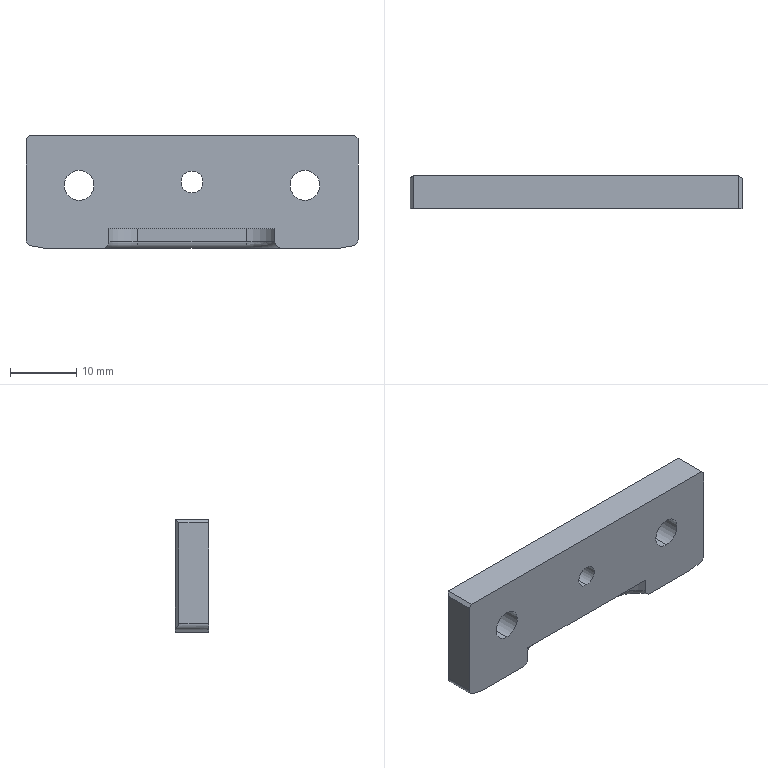Part | NX | features BREP 1 | 1 solid | 27 faces | box 50 x 5 x 17 mm | volume 3859 mm3 | plane 14 | cylinder 11 | torus 2 | commonest cylinder face diameters 4.5 x4 2 x3 3.3 x2 10 x2
STEP:
#1=CARTESIAN_POINT('',(0.,0.,8.35));
#2=VERTEX_POINT('',#1);
#3=CARTESIAN_POINT('',(0.,0.,11.65));
#4=VERTEX_POINT('',#3);
#5=CARTESIAN_POINT('',(0.,0.,10.));
#6=DIRECTION('',(0.,1.,0.));
#7=DIRECTION('',(0.,0.,1.));
#8=AXIS2_PLACEMENT_3D('',#5,#6,#7);
#9=CIRCLE('',#8,1.65);
#10=EDGE_CURVE('',#2,#4,#9,.T.);
#11=ORIENTED_EDGE('',*,*,#10,.F.);
#12=CARTESIAN_POINT('',(0.,5.,8.35));
#13=VERTEX_POINT('',#12);
#14=CARTESIAN_POINT('',(0.,5.,8.35));
#15=DIRECTION('',(0.,1.,0.));
#16=VECTOR('',#15,1000.);
#17=LINE('',#14,#16);
#18=EDGE_CURVE('',#13,#2,#17,.F.);
#19=ORIENTED_EDGE('',*,*,#18,.F.);
#20=CARTESIAN_POINT('',(0.,5.,11.65));
#21=VERTEX_POINT('',#20);
#22=CARTESIAN_POINT('',(0.,5.,10.));
#23=DIRECTION('',(0.,1.,0.));
#24=DIRECTION('',(0.,0.,1.));
#25=AXIS2_PLACEMENT_3D('',#22,#23,#24);
#26=CIRCLE('',#25,1.65);
#27=EDGE_CURVE('',#13,#21,#26,.T.);
#28=ORIENTED_EDGE('',*,*,#27,.T.);
#29=CARTESIAN_POINT('',(0.,5.,11.65));
#30=DIRECTION('',(0.,1.,0.));
#31=VECTOR('',#30,1000.);
#32=LINE('',#29,#31);
#33=EDGE_CURVE('',#21,#4,#32,.F.);
#34=ORIENTED_EDGE('',*,*,#33,.T.);
#35=EDGE_LOOP('',(#11,#19,#28,#34));
#36=FACE_BOUND('',#35,.T.);
#37=CARTESIAN_POINT('',(0.,5.,10.));
#38=DIRECTION('',(0.,1.,0.));
#39=DIRECTION('',(0.,0.,1.));
#40=AXIS2_PLACEMENT_3D('',#37,#38,#39);
#41=CYLINDRICAL_SURFACE('',#40,1.65);
#42=ADVANCED_FACE('',(#36),#41,.F.);
#43=CARTESIAN_POINT('',(17.,0.,7.25));
#44=VERTEX_POINT('',#43);
#45=CARTESIAN_POINT('',(17.,0.,11.75));
#46=VERTEX_POINT('',#45);
#47=CARTESIAN_POINT('',(17.,0.,9.5));
#48=DIRECTION('',(0.,1.,0.));
#49=DIRECTION('',(0.,0.,1.));
#50=AXIS2_PLACEMENT_3D('',#47,#48,#49);
#51=CIRCLE('',#50,2.25);
#52=EDGE_CURVE('',#44,#46,#51,.T.);
#53=ORIENTED_EDGE('',*,*,#52,.F.);
#54=CARTESIAN_POINT('',(17.,5.,7.25));
#55=VERTEX_POINT('',#54);
#56=CARTESIAN_POINT('',(17.,5.,7.25));
#57=DIRECTION('',(0.,1.,0.));
#58=VECTOR('',#57,1000.);
#59=LINE('',#56,#58);
#60=EDGE_CURVE('',#55,#44,#59,.F.);
#61=ORIENTED_EDGE('',*,*,#60,.F.);
#62=CARTESIAN_POINT('',(17.,5.,11.75));
#63=VERTEX_POINT('',#62);
#64=CARTESIAN_POINT('',(17.,5.,9.5));
#65=DIRECTION('',(0.,1.,0.));
#66=DIRECTION('',(0.,0.,1.));
#67=AXIS2_PLACEMENT_3D('',#64,#65,#66);
#68=CIRCLE('',#67,2.25);
#69=EDGE_CURVE('',#55,#63,#68,.T.);
#70=ORIENTED_EDGE('',*,*,#69,.T.);
#71=CARTESIAN_POINT('',(17.,5.,11.75));
#72=DIRECTION('',(0.,1.,0.));
#73=VECTOR('',#72,1000.);
#74=LINE('',#71,#73);
#75=EDGE_CURVE('',#63,#46,#74,.F.);
#76=ORIENTED_EDGE('',*,*,#75,.T.);
#77=EDGE_LOOP('',(#53,#61,#70,#76));
#78=FACE_BOUND('',#77,.T.);
#79=CARTESIAN_POINT('',(17.,5.,9.5));
#80=DIRECTION('',(0.,1.,0.));
#81=DIRECTION('',(0.,0.,1.));
#82=AXIS2_PLACEMENT_3D('',#79,#80,#81);
#83=CYLINDRICAL_SURFACE('',#82,2.25);
#84=ADVANCED_FACE('',(#78),#83,.F.);
#85=CARTESIAN_POINT('',(-17.,0.,7.25));
#86=VERTEX_POINT('',#85);
#87=CARTESIAN_POINT('',(-17.,0.,11.75));
#88=VERTEX_POINT('',#87);
#89=CARTESIAN_POINT('',(-17.,0.,9.5));
#90=DIRECTION('',(0.,1.,0.));
#91=DIRECTION('',(0.,0.,1.));
#92=AXIS2_PLACEMENT_3D('',#89,#90,#91);
#93=CIRCLE('',#92,2.25);
#94=EDGE_CURVE('',#86,#88,#93,.T.);
#95=ORIENTED_EDGE('',*,*,#94,.F.);
#96=CARTESIAN_POINT('',(-17.,5.,7.25));
#97=VERTEX_POINT('',#96);
#98=CARTESIAN_POINT('',(-17.,5.,7.25));
#99=DIRECTION('',(0.,1.,0.));
#100=VECTOR('',#99,1000.);
#101=LINE('',#98,#100);
#102=EDGE_CURVE('',#97,#86,#101,.F.);
#103=ORIENTED_EDGE('',*,*,#102,.F.);
#104=CARTESIAN_POINT('',(-17.,5.,11.75));
#105=VERTEX_POINT('',#104);
#106=CARTESIAN_POINT('',(-17.,5.,9.5));
#107=DIRECTION('',(0.,1.,0.));
#108=DIRECTION('',(0.,0.,1.));
#109=AXIS2_PLACEMENT_3D('',#106,#107,#108);
#110=CIRCLE('',#109,2.25);
#111=EDGE_CURVE('',#97,#105,#110,.T.);
#112=ORIENTED_EDGE('',*,*,#111,.T.);
#113=CARTESIAN_POINT('',(-17.,5.,11.75));
#114=DIRECTION('',(0.,1.,0.));
#115=VECTOR('',#114,1000.);
#116=LINE('',#113,#115);
#117=EDGE_CURVE('',#105,#88,#116,.F.);
#118=ORIENTED_EDGE('',*,*,#117,.T.);
#119=EDGE_LOOP('',(#95,#103,#112,#118));
#120=FACE_BOUND('',#119,.T.);
#121=CARTESIAN_POINT('',(-17.,5.,9.5));
#122=DIRECTION('',(0.,1.,0.));
#123=DIRECTION('',(0.,0.,1.));
#124=AXIS2_PLACEMENT_3D('',#121,#122,#123);
#125=CYLINDRICAL_SURFACE('',#124,2.25);
#126=ADVANCED_FACE('',(#120),#125,.F.);
#127=CARTESIAN_POINT('',(-25.,0.,16.5));
#128=VERTEX_POINT('',#127);
#129=CARTESIAN_POINT('',(-25.,4.5,16.5));
#130=VERTEX_POINT('',#129);
#131=CARTESIAN_POINT('',(-25.,5.,16.5));
#132=DIRECTION('',(0.,1.,0.));
#133=VECTOR('',#132,1000.);
#134=LINE('',#131,#133);
#135=EDGE_CURVE('',#128,#130,#134,.T.);
#136=ORIENTED_EDGE('',*,*,#135,.T.);
#137=CARTESIAN_POINT('',(-25.,4.5,1.368));
#138=VERTEX_POINT('',#137);
#139=CARTESIAN_POINT('',(-25.,4.5,17.));
#140=DIRECTION('',(0.,0.,-1.));
#141=VECTOR('',#140,1000.);
#142=LINE('',#139,#141);
#143=EDGE_CURVE('',#130,#138,#142,.T.);
#144=ORIENTED_EDGE('',*,*,#143,.T.);
#145=CARTESIAN_POINT('',(-25.,0.,1.368));
#146=VERTEX_POINT('',#145);
#147=CARTESIAN_POINT('',(-25.,0.,1.368));
#148=DIRECTION('',(0.,-1.,0.));
#149=VECTOR('',#148,1000.);
#150=LINE('',#147,#149);
#151=EDGE_CURVE('',#138,#146,#150,.T.);
#152=ORIENTED_EDGE('',*,*,#151,.T.);
#153=CARTESIAN_POINT('',(-25.,0.,2.));
#154=DIRECTION('',(0.,0.,-1.));
#155=VECTOR('',#154,1000.);
#156=LINE('',#153,#155);
#157=EDGE_CURVE('',#128,#146,#156,.T.);
#158=ORIENTED_EDGE('',*,*,#157,.F.);
#159=EDGE_LOOP('',(#136,#144,#152,#158));
#160=FACE_BOUND('',#159,.T.);
#161=CARTESIAN_POINT('',(-25.,5.,2.));
#162=DIRECTION('',(1.,0.,0.));
#163=DIRECTION('',(0.,-1.,0.));
#164=AXIS2_PLACEMENT_3D('',#161,#162,#163);
#165=PLANE('',#164);
#166=ADVANCED_FACE('',(#160),#165,.F.);
#167=CARTESIAN_POINT('',(-22.,0.,0.));
#168=VERTEX_POINT('',#167);
#169=CARTESIAN_POINT('',(-13.624,0.,0.));
#170=VERTEX_POINT('',#169);
#171=CARTESIAN_POINT('',(-25.,0.,0.));
#172=DIRECTION('',(1.,0.,0.));
#173=VECTOR('',#172,1000.);
#174=LINE('',#171,#173);
#175=EDGE_CURVE('',#168,#170,#174,.T.);
#176=ORIENTED_EDGE('',*,*,#175,.T.);
#177=CARTESIAN_POINT('',(-12.5,0.,1.));
#178=VERTEX_POINT('',#177);
#179=CARTESIAN_POINT('',(-13.624,0.,0.));
#180=CARTESIAN_POINT('',(-13.065,0.,0.));
#181=CARTESIAN_POINT('',(-12.5,0.,0.4402));
#182=CARTESIAN_POINT('',(-12.5,0.,1.));
#183=B_SPLINE_CURVE_WITH_KNOTS('',3,(#179,#180,#181,#182),.UNSPECIFIED.,.F.,.F.,(4,4),(0.,1.),.UNSPECIFIED.);
#184=EDGE_CURVE('',#170,#178,#183,.T.);
#185=ORIENTED_EDGE('',*,*,#184,.T.);
#186=CARTESIAN_POINT('',(-12.5,0.,3.));
#187=VERTEX_POINT('',#186);
#188=CARTESIAN_POINT('',(-12.5,0.,3.));
#189=DIRECTION('',(0.,0.,-1.));
#190=VECTOR('',#189,1000.);
#191=LINE('',#188,#190);
#192=EDGE_CURVE('',#187,#178,#191,.T.);
#193=ORIENTED_EDGE('',*,*,#192,.F.);
#194=CARTESIAN_POINT('',(12.5,0.,3.));
#195=VERTEX_POINT('',#194);
#196=CARTESIAN_POINT('',(12.5,0.,3.));
#197=DIRECTION('',(-1.,0.,0.));
#198=VECTOR('',#197,1000.);
#199=LINE('',#196,#198);
#200=EDGE_CURVE('',#195,#187,#199,.T.);
#201=ORIENTED_EDGE('',*,*,#200,.F.);
#202=CARTESIAN_POINT('',(12.5,0.,1.));
#203=VERTEX_POINT('',#202);
#204=CARTESIAN_POINT('',(12.5,0.,3.));
#205=DIRECTION('',(0.,0.,-1.));
#206=VECTOR('',#205,1000.);
#207=LINE('',#204,#206);
#208=EDGE_CURVE('',#195,#203,#207,.T.);
#209=ORIENTED_EDGE('',*,*,#208,.T.);
#210=CARTESIAN_POINT('',(13.624,0.,0.));
#211=VERTEX_POINT('',#210);
#212=CARTESIAN_POINT('',(12.5,0.,1.));
#213=CARTESIAN_POINT('',(12.5,0.,0.444));
#214=CARTESIAN_POINT('',(13.062,0.,0.));
#215=CARTESIAN_POINT('',(13.624,0.,0.));
#216=B_SPLINE_CURVE_WITH_KNOTS('',3,(#212,#213,#214,#215),.UNSPECIFIED.,.F.,.F.,(4,4),(0.,1.),.UNSPECIFIED.);
#217=EDGE_CURVE('',#203,#211,#216,.T.);
#218=ORIENTED_EDGE('',*,*,#217,.T.);
#219=CARTESIAN_POINT('',(22.,0.,0.));
#220=VERTEX_POINT('',#219);
#221=CARTESIAN_POINT('',(-25.,0.,0.));
#222=DIRECTION('',(1.,0.,0.));
#223=VECTOR('',#222,1000.);
#224=LINE('',#221,#223);
#225=EDGE_CURVE('',#211,#220,#224,.T.);
#226=ORIENTED_EDGE('',*,*,#225,.T.);
#227=CARTESIAN_POINT('',(24.174,0.,0.3833));
#228=VERTEX_POINT('',#227);
#229=CARTESIAN_POINT('',(25.,0.,0.529));
#230=DIRECTION('',(0.9848,0.,0.1736));
#231=VECTOR('',#230,1000.);
#232=LINE('',#229,#231);
#233=EDGE_CURVE('',#220,#228,#232,.T.);
#234=ORIENTED_EDGE('',*,*,#233,.T.);
#235=CARTESIAN_POINT('',(25.,0.,1.368));
#236=VERTEX_POINT('',#235);
#237=CARTESIAN_POINT('',(24.,0.,1.368));
#238=DIRECTION('',(0.,-1.,0.));
#239=DIRECTION('',(0.,0.,1.));
#240=AXIS2_PLACEMENT_3D('',#237,#238,#239);
#241=CIRCLE('',#240,1.);
#242=EDGE_CURVE('',#228,#236,#241,.T.);
#243=ORIENTED_EDGE('',*,*,#242,.T.);
#244=CARTESIAN_POINT('',(25.,0.,16.5));
#245=VERTEX_POINT('',#244);
#246=CARTESIAN_POINT('',(25.,0.,2.));
#247=DIRECTION('',(0.,0.,-1.));
#248=VECTOR('',#247,1000.);
#249=LINE('',#246,#248);
#250=EDGE_CURVE('',#245,#236,#249,.T.);
#251=ORIENTED_EDGE('',*,*,#250,.F.);
#252=CARTESIAN_POINT('',(24.5,0.,17.));
#253=VERTEX_POINT('',#252);
#254=CARTESIAN_POINT('',(24.5,0.,17.));
#255=DIRECTION('',(-0.7071,0.,0.7071));
#256=VECTOR('',#255,1000.);
#257=LINE('',#254,#256);
#258=EDGE_CURVE('',#245,#253,#257,.T.);
#259=ORIENTED_EDGE('',*,*,#258,.T.);
#260=CARTESIAN_POINT('',(-24.5,0.,17.));
#261=VERTEX_POINT('',#260);
#262=CARTESIAN_POINT('',(-25.,0.,17.));
#263=DIRECTION('',(1.,0.,0.));
#264=VECTOR('',#263,1000.);
#265=LINE('',#262,#264);
#266=EDGE_CURVE('',#261,#253,#265,.T.);
#267=ORIENTED_EDGE('',*,*,#266,.F.);
#268=CARTESIAN_POINT('',(-24.5,0.,17.));
#269=DIRECTION('',(-0.7071,0.,-0.7071));
#270=VECTOR('',#269,1000.);
#271=LINE('',#268,#270);
#272=EDGE_CURVE('',#261,#128,#271,.T.);
#273=ORIENTED_EDGE('',*,*,#272,.T.);
#274=ORIENTED_EDGE('',*,*,#157,.T.);
#275=CARTESIAN_POINT('',(-24.174,0.,0.3833));
#276=VERTEX_POINT('',#275);
#277=CARTESIAN_POINT('',(-24.,0.,1.368));
#278=DIRECTION('',(0.,-1.,0.));
#279=DIRECTION('',(0.,0.,1.));
#280=AXIS2_PLACEMENT_3D('',#277,#278,#279);
#281=CIRCLE('',#280,1.);
#282=EDGE_CURVE('',#146,#276,#281,.T.);
#283=ORIENTED_EDGE('',*,*,#282,.T.);
#284=CARTESIAN_POINT('',(-25.,0.,0.529));
#285=DIRECTION('',(0.9848,0.,-0.1736));
#286=VECTOR('',#285,1000.);
#287=LINE('',#284,#286);
#288=EDGE_CURVE('',#276,#168,#287,.T.);
#289=ORIENTED_EDGE('',*,*,#288,.T.);
#290=EDGE_LOOP('',(#176,#185,#193,#201,#209,#218,#226,#234,#243,#251,#259,#267,#273,#274,#283,#289));
#291=FACE_BOUND('',#290,.T.);
#292=CARTESIAN_POINT('',(0.,0.,10.));
#293=DIRECTION('',(0.,1.,0.));
#294=DIRECTION('',(0.,0.,1.));
#295=AXIS2_PLACEMENT_3D('',#292,#293,#294);
#296=CIRCLE('',#295,1.65);
#297=EDGE_CURVE('',#4,#2,#296,.T.);
#298=ORIENTED_EDGE('',*,*,#297,.T.);
#299=ORIENTED_EDGE('',*,*,#10,.T.);
#300=EDGE_LOOP('',(#298,#299));
#301=FACE_BOUND('',#300,.T.);
#302=CARTESIAN_POINT('',(17.,0.,9.5));
#303=DIRECTION('',(0.,1.,0.));
#304=DIRECTION('',(0.,0.,1.));
#305=AXIS2_PLACEMENT_3D('',#302,#303,#304);
#306=CIRCLE('',#305,2.25);
#307=EDGE_CURVE('',#46,#44,#306,.T.);
#308=ORIENTED_EDGE('',*,*,#307,.T.);
#309=ORIENTED_EDGE('',*,*,#52,.T.);
#310=EDGE_LOOP('',(#308,#309));
#311=FACE_BOUND('',#310,.T.);
#312=CARTESIAN_POINT('',(-17.,0.,9.5));
#313=DIRECTION('',(0.,1.,0.));
#314=DIRECTION('',(0.,0.,1.));
#315=AXIS2_PLACEMENT_3D('',#312,#313,#314);
#316=CIRCLE('',#315,2.25);
#317=EDGE_CURVE('',#88,#86,#316,.T.);
#318=ORIENTED_EDGE('',*,*,#317,.T.);
#319=ORIENTED_EDGE('',*,*,#94,.T.);
#320=EDGE_LOOP('',(#318,#319));
#321=FACE_BOUND('',#320,.T.);
#322=CARTESIAN_POINT('',(-25.,0.,2.));
#323=DIRECTION('',(0.,1.,0.));
#324=DIRECTION('',(1.,0.,0.));
#325=AXIS2_PLACEMENT_3D('',#322,#323,#324);
#326=PLANE('',#325);
#327=ADVANCED_FACE('',(#291,#301,#311,#321),#326,.F.);
#328=CARTESIAN_POINT('',(25.,4.5,1.368));
#329=VERTEX_POINT('',#328);
#330=CARTESIAN_POINT('',(25.,5.,1.368));
#331=DIRECTION('',(0.,1.,0.));
#332=VECTOR('',#331,1000.);
#333=LINE('',#330,#332);
#334=EDGE_CURVE('',#236,#329,#333,.T.);
#335=ORIENTED_EDGE('',*,*,#334,.T.);
#336=CARTESIAN_POINT('',(25.,4.5,16.5));
#337=VERTEX_POINT('',#336);
#338=CARTESIAN_POINT('',(25.,4.5,17.));
#339=DIRECTION('',(0.,0.,-1.));
#340=VECTOR('',#339,1000.);
#341=LINE('',#338,#340);
#342=EDGE_CURVE('',#337,#329,#341,.T.);
#343=ORIENTED_EDGE('',*,*,#342,.F.);
#344=CARTESIAN_POINT('',(25.,5.,16.5));
#345=DIRECTION('',(0.,-1.,0.));
#346=VECTOR('',#345,1000.);
#347=LINE('',#344,#346);
#348=EDGE_CURVE('',#337,#245,#347,.T.);
#349=ORIENTED_EDGE('',*,*,#348,.T.);
#350=ORIENTED_EDGE('',*,*,#250,.T.);
#351=EDGE_LOOP('',(#335,#343,#349,#350));
#352=FACE_BOUND('',#351,.T.);
#353=CARTESIAN_POINT('',(25.,5.,2.));
#354=DIRECTION('',(-1.,0.,0.));
#355=DIRECTION('',(0.,1.,0.));
#356=AXIS2_PLACEMENT_3D('',#353,#354,#355);
#357=PLANE('',#356);
#358=ADVANCED_FACE('',(#352),#357,.F.);
#359=CARTESIAN_POINT('',(-24.174,5.,0.3833));
#360=VERTEX_POINT('',#359);
#361=CARTESIAN_POINT('',(-24.5,5.,0.5021));
#362=VERTEX_POINT('',#361);
#363=CARTESIAN_POINT('',(-24.,5.,1.368));
#364=DIRECTION('',(0.,1.,0.));
#365=DIRECTION('',(1.,0.,0.));
#366=AXIS2_PLACEMENT_3D('',#363,#364,#365);
#367=CIRCLE('',#366,1.);
#368=EDGE_CURVE('',#360,#362,#367,.T.);
#369=ORIENTED_EDGE('',*,*,#368,.T.);
#370=CARTESIAN_POINT('',(-24.5,5.,17.));
#371=VERTEX_POINT('',#370);
#372=CARTESIAN_POINT('',(-24.5,5.,17.));
#373=DIRECTION('',(0.,0.,-1.));
#374=VECTOR('',#373,1000.);
#375=LINE('',#372,#374);
#376=EDGE_CURVE('',#371,#362,#375,.T.);
#377=ORIENTED_EDGE('',*,*,#376,.F.);
#378=CARTESIAN_POINT('',(24.5,5.,17.));
#379=VERTEX_POINT('',#378);
#380=CARTESIAN_POINT('',(-25.,5.,17.));
#381=DIRECTION('',(-1.,0.,0.));
#382=VECTOR('',#381,1000.);
#383=LINE('',#380,#382);
#384=EDGE_CURVE('',#379,#371,#383,.T.);
#385=ORIENTED_EDGE('',*,*,#384,.F.);
#386=CARTESIAN_POINT('',(24.5,5.,0.5021));
#387=VERTEX_POINT('',#386);
#388=CARTESIAN_POINT('',(24.5,5.,17.));
#389=DIRECTION('',(0.,0.,-1.));
#390=VECTOR('',#389,1000.);
#391=LINE('',#388,#390);
#392=EDGE_CURVE('',#379,#387,#391,.T.);
#393=ORIENTED_EDGE('',*,*,#392,.T.);
#394=CARTESIAN_POINT('',(24.174,5.,0.3833));
#395=VERTEX_POINT('',#394);
#396=CARTESIAN_POINT('',(24.,5.,1.368));
#397=DIRECTION('',(0.,1.,0.));
#398=DIRECTION('',(1.,0.,0.));
#399=AXIS2_PLACEMENT_3D('',#396,#397,#398);
#400=CIRCLE('',#399,1.);
#401=EDGE_CURVE('',#387,#395,#400,.T.);
#402=ORIENTED_EDGE('',*,*,#401,.T.);
#403=CARTESIAN_POINT('',(22.,5.,0.));
#404=VERTEX_POINT('',#403);
#405=CARTESIAN_POINT('',(25.,5.,0.529));
#406=DIRECTION('',(-0.9848,0.,-0.1736));
#407=VECTOR('',#406,1000.);
#408=LINE('',#405,#407);
#409=EDGE_CURVE('',#395,#404,#408,.T.);
#410=ORIENTED_EDGE('',*,*,#409,.T.);
#411=CARTESIAN_POINT('',(-22.,5.,0.));
#412=VERTEX_POINT('',#411);
#413=CARTESIAN_POINT('',(-25.,5.,0.));
#414=DIRECTION('',(-1.,0.,0.));
#415=VECTOR('',#414,1000.);
#416=LINE('',#413,#415);
#417=EDGE_CURVE('',#404,#412,#416,.T.);
#418=ORIENTED_EDGE('',*,*,#417,.T.);
#419=CARTESIAN_POINT('',(-25.,5.,0.529));
#420=DIRECTION('',(-0.9848,0.,0.1736));
#421=VECTOR('',#420,1000.);
#422=LINE('',#419,#421);
#423=EDGE_CURVE('',#412,#360,#422,.T.);
#424=ORIENTED_EDGE('',*,*,#423,.T.);
#425=EDGE_LOOP('',(#369,#377,#385,#393,#402,#410,#418,#424));
#426=FACE_BOUND('',#425,.T.);
#427=CARTESIAN_POINT('',(0.,5.,10.));
#428=DIRECTION('',(0.,1.,0.));
#429=DIRECTION('',(0.,0.,1.));
#430=AXIS2_PLACEMENT_3D('',#427,#428,#429);
#431=CIRCLE('',#430,1.65);
#432=EDGE_CURVE('',#21,#13,#431,.T.);
#433=ORIENTED_EDGE('',*,*,#432,.F.);
#434=ORIENTED_EDGE('',*,*,#27,.F.);
#435=EDGE_LOOP('',(#433,#434));
#436=FACE_BOUND('',#435,.T.);
#437=CARTESIAN_POINT('',(17.,5.,9.5));
#438=DIRECTION('',(0.,1.,0.));
#439=DIRECTION('',(0.,0.,1.));
#440=AXIS2_PLACEMENT_3D('',#437,#438,#439);
#441=CIRCLE('',#440,2.25);
#442=EDGE_CURVE('',#63,#55,#441,.T.);
#443=ORIENTED_EDGE('',*,*,#442,.F.);
#444=ORIENTED_EDGE('',*,*,#69,.F.);
#445=EDGE_LOOP('',(#443,#444));
#446=FACE_BOUND('',#445,.T.);
#447=CARTESIAN_POINT('',(-17.,5.,9.5));
#448=DIRECTION('',(0.,1.,0.));
#449=DIRECTION('',(0.,0.,1.));
#450=AXIS2_PLACEMENT_3D('',#447,#448,#449);
#451=CIRCLE('',#450,2.25);
#452=EDGE_CURVE('',#105,#97,#451,.T.);
#453=ORIENTED_EDGE('',*,*,#452,.F.);
#454=ORIENTED_EDGE('',*,*,#111,.F.);
#455=EDGE_LOOP('',(#453,#454));
#456=FACE_BOUND('',#455,.T.);
#457=CARTESIAN_POINT('',(-25.,5.,2.));
#458=DIRECTION('',(0.,-1.,0.));
#459=DIRECTION('',(-1.,0.,0.));
#460=AXIS2_PLACEMENT_3D('',#457,#458,#459);
#461=PLANE('',#460);
#462=ADVANCED_FACE('',(#426,#436,#446,#456),#461,.F.);
#463=CARTESIAN_POINT('',(8.17,3.5,0.));
#464=VERTEX_POINT('',#463);
#465=CARTESIAN_POINT('',(-8.17,3.5,0.));
#466=VERTEX_POINT('',#465);
#467=CARTESIAN_POINT('',(-25.,3.5,0.));
#468=DIRECTION('',(-1.,0.,0.));
#469=VECTOR('',#468,1000.);
#470=LINE('',#467,#469);
#471=EDGE_CURVE('',#464,#466,#470,.T.);
#472=ORIENTED_EDGE('',*,*,#471,.T.);
#473=CARTESIAN_POINT('',(-8.17,-2.5,0.));
#474=DIRECTION('',(0.,0.,1.));
#475=DIRECTION('',(1.,0.,0.));
#476=AXIS2_PLACEMENT_3D('',#473,#474,#475);
#477=CIRCLE('',#476,6.);
#478=EDGE_CURVE('',#466,#170,#477,.T.);
#479=ORIENTED_EDGE('',*,*,#478,.T.);
#480=ORIENTED_EDGE('',*,*,#175,.F.);
#481=CARTESIAN_POINT('',(-22.,5.,0.));
#482=DIRECTION('',(0.,1.,0.));
#483=VECTOR('',#482,1000.);
#484=LINE('',#481,#483);
#485=EDGE_CURVE('',#168,#412,#484,.T.);
#486=ORIENTED_EDGE('',*,*,#485,.T.);
#487=ORIENTED_EDGE('',*,*,#417,.F.);
#488=CARTESIAN_POINT('',(22.,5.,0.));
#489=DIRECTION('',(0.,-1.,0.));
#490=VECTOR('',#489,1000.);
#491=LINE('',#488,#490);
#492=EDGE_CURVE('',#404,#220,#491,.T.);
#493=ORIENTED_EDGE('',*,*,#492,.T.);
#494=ORIENTED_EDGE('',*,*,#225,.F.);
#495=CARTESIAN_POINT('',(8.17,-2.5,0.));
#496=DIRECTION('',(0.,0.,1.));
#497=DIRECTION('',(1.,0.,0.));
#498=AXIS2_PLACEMENT_3D('',#495,#496,#497);
#499=CIRCLE('',#498,6.);
#500=EDGE_CURVE('',#211,#464,#499,.T.);
#501=ORIENTED_EDGE('',*,*,#500,.T.);
#502=EDGE_LOOP('',(#472,#479,#480,#486,#487,#493,#494,#501));
#503=FACE_BOUND('',#502,.T.);
#504=CARTESIAN_POINT('',(-25.,5.,0.));
#505=DIRECTION('',(0.,0.,1.));
#506=DIRECTION('',(1.,0.,0.));
#507=AXIS2_PLACEMENT_3D('',#504,#505,#506);
#508=PLANE('',#507);
#509=ADVANCED_FACE('',(#503),#508,.F.);
#510=ORIENTED_EDGE('',*,*,#384,.T.);
#511=CARTESIAN_POINT('',(-24.5,5.,17.));
#512=DIRECTION('',(0.,-1.,0.));
#513=VECTOR('',#512,1000.);
#514=LINE('',#511,#513);
#515=EDGE_CURVE('',#371,#261,#514,.T.);
#516=ORIENTED_EDGE('',*,*,#515,.T.);
#517=ORIENTED_EDGE('',*,*,#266,.T.);
#518=CARTESIAN_POINT('',(24.5,5.,17.));
#519=DIRECTION('',(0.,1.,0.));
#520=VECTOR('',#519,1000.);
#521=LINE('',#518,#520);
#522=EDGE_CURVE('',#253,#379,#521,.T.);
#523=ORIENTED_EDGE('',*,*,#522,.T.);
#524=EDGE_LOOP('',(#510,#516,#517,#523));
#525=FACE_BOUND('',#524,.T.);
#526=CARTESIAN_POINT('',(-25.,5.,17.));
#527=DIRECTION('',(0.,0.,-1.));
#528=DIRECTION('',(0.,-1.,0.));
#529=AXIS2_PLACEMENT_3D('',#526,#527,#528);
#530=PLANE('',#529);
#531=ADVANCED_FACE('',(#525),#530,.F.);
#532=ORIENTED_EDGE('',*,*,#102,.T.);
#533=ORIENTED_EDGE('',*,*,#317,.F.);
#534=ORIENTED_EDGE('',*,*,#117,.F.);
#535=ORIENTED_EDGE('',*,*,#452,.T.);
#536=EDGE_LOOP('',(#532,#533,#534,#535));
#537=FACE_BOUND('',#536,.T.);
#538=CARTESIAN_POINT('',(-17.,5.,9.5));
#539=DIRECTION('',(0.,1.,0.));
#540=DIRECTION('',(0.,0.,1.));
#541=AXIS2_PLACEMENT_3D('',#538,#539,#540);
#542=CYLINDRICAL_SURFACE('',#541,2.25);
#543=ADVANCED_FACE('',(#537),#542,.F.);
#544=ORIENTED_EDGE('',*,*,#60,.T.);
#545=ORIENTED_EDGE('',*,*,#307,.F.);
#546=ORIENTED_EDGE('',*,*,#75,.F.);
#547=ORIENTED_EDGE('',*,*,#442,.T.);
#548=EDGE_LOOP('',(#544,#545,#546,#547));
#549=FACE_BOUND('',#548,.T.);
#550=CARTESIAN_POINT('',(17.,5.,9.5));
#551=DIRECTION('',(0.,1.,0.));
#552=DIRECTION('',(0.,0.,1.));
#553=AXIS2_PLACEMENT_3D('',#550,#551,#552);
#554=CYLINDRICAL_SURFACE('',#553,2.25);
#555=ADVANCED_FACE('',(#549),#554,.F.);
#556=CARTESIAN_POINT('',(-24.5,5.,17.));
#557=DIRECTION('',(0.5774,0.5774,0.5774));
#558=VECTOR('',#557,1000.);
#559=LINE('',#556,#558);
#560=EDGE_CURVE('',#130,#371,#559,.T.);
#561=ORIENTED_EDGE('',*,*,#560,.F.);
#562=ORIENTED_EDGE('',*,*,#135,.F.);
#563=ORIENTED_EDGE('',*,*,#272,.F.);
#564=ORIENTED_EDGE('',*,*,#515,.F.);
#565=EDGE_LOOP('',(#561,#562,#563,#564));
#566=FACE_BOUND('',#565,.T.);
#567=CARTESIAN_POINT('',(-24.5,5.,17.));
#568=DIRECTION('',(0.7071,0.,-0.7071));
#569=DIRECTION('',(0.,-1.,0.));
#570=AXIS2_PLACEMENT_3D('',#567,#568,#569);
#571=PLANE('',#570);
#572=ADVANCED_FACE('',(#566),#571,.F.);
#573=CARTESIAN_POINT('',(24.5,5.,17.));
#574=DIRECTION('',(0.5774,-0.5774,-0.5774));
#575=VECTOR('',#574,1000.);
#576=LINE('',#573,#575);
#577=EDGE_CURVE('',#379,#337,#576,.T.);
#578=ORIENTED_EDGE('',*,*,#577,.F.);
#579=ORIENTED_EDGE('',*,*,#522,.F.);
#580=ORIENTED_EDGE('',*,*,#258,.F.);
#581=ORIENTED_EDGE('',*,*,#348,.F.);
#582=EDGE_LOOP('',(#578,#579,#580,#581));
#583=FACE_BOUND('',#582,.T.);
#584=CARTESIAN_POINT('',(24.5,5.,17.));
#585=DIRECTION('',(-0.7071,0.,-0.7071));
#586=DIRECTION('',(-0.7071,0.,0.7071));
#587=AXIS2_PLACEMENT_3D('',#584,#585,#586);
#588=PLANE('',#587);
#589=ADVANCED_FACE('',(#583),#588,.F.);
#590=ORIENTED_EDGE('',*,*,#288,.F.);
#591=CARTESIAN_POINT('',(-24.174,5.,0.3833));
#592=DIRECTION('',(0.,1.,0.));
#593=VECTOR('',#592,1000.);
#594=LINE('',#591,#593);
#595=EDGE_CURVE('',#276,#360,#594,.T.);
#596=ORIENTED_EDGE('',*,*,#595,.T.);
#597=ORIENTED_EDGE('',*,*,#423,.F.);
#598=ORIENTED_EDGE('',*,*,#485,.F.);
#599=EDGE_LOOP('',(#590,#596,#597,#598));
#600=FACE_BOUND('',#599,.T.);
#601=CARTESIAN_POINT('',(-25.,5.,0.529));
#602=DIRECTION('',(0.1736,0.,0.9848));
#603=DIRECTION('',(0.,-1.,0.));
#604=AXIS2_PLACEMENT_3D('',#601,#602,#603);
#605=PLANE('',#604);
#606=ADVANCED_FACE('',(#600),#605,.F.);
#607=ORIENTED_EDGE('',*,*,#409,.F.);
#608=CARTESIAN_POINT('',(24.174,0.,0.3833));
#609=DIRECTION('',(0.,-1.,0.));
#610=VECTOR('',#609,1000.);
#611=LINE('',#608,#610);
#612=EDGE_CURVE('',#395,#228,#611,.T.);
#613=ORIENTED_EDGE('',*,*,#612,.T.);
#614=ORIENTED_EDGE('',*,*,#233,.F.);
#615=ORIENTED_EDGE('',*,*,#492,.F.);
#616=EDGE_LOOP('',(#607,#613,#614,#615));
#617=FACE_BOUND('',#616,.T.);
#618=CARTESIAN_POINT('',(25.,5.,0.529));
#619=DIRECTION('',(-0.1736,0.,0.9848));
#620=DIRECTION('',(0.,1.,0.));
#621=AXIS2_PLACEMENT_3D('',#618,#619,#620);
#622=PLANE('',#621);
#623=ADVANCED_FACE('',(#617),#622,.F.);
#624=CARTESIAN_POINT('',(25.,4.5,1.368));
#625=CARTESIAN_POINT('',(25.,4.5,1.002));
#626=CARTESIAN_POINT('',(24.817,4.683,0.6851));
#627=CARTESIAN_POINT('',(24.5,5.,0.5021));
#628=(BOUNDED_CURVE()B_SPLINE_CURVE(3,(#624,#625,#626,#627),.UNSPECIFIED.,.F.,.F.)B_SPLINE_CURVE_WITH_KNOTS((4,4),(3.142,4.189),.UNSPECIFIED.)CURVE()GEOMETRIC_REPRESENTATION_ITEM()RATIONAL_B_SPLINE_CURVE((1.,0.9107,0.9107,1.))REPRESENTATION_ITEM(''));
#629=EDGE_CURVE('',#329,#387,#628,.T.);
#630=ORIENTED_EDGE('',*,*,#629,.F.);
#631=ORIENTED_EDGE('',*,*,#334,.F.);
#632=ORIENTED_EDGE('',*,*,#242,.F.);
#633=ORIENTED_EDGE('',*,*,#612,.F.);
#634=ORIENTED_EDGE('',*,*,#401,.F.);
#635=EDGE_LOOP('',(#630,#631,#632,#633,#634));
#636=FACE_BOUND('',#635,.T.);
#637=CARTESIAN_POINT('',(24.,5.,1.368));
#638=DIRECTION('',(0.,1.,0.));
#639=DIRECTION('',(-1.,0.,0.));
#640=AXIS2_PLACEMENT_3D('',#637,#638,#639);
#641=CYLINDRICAL_SURFACE('',#640,1.);
#642=ADVANCED_FACE('',(#636),#641,.T.);
#643=CARTESIAN_POINT('',(-24.5,5.,0.5021));
#644=CARTESIAN_POINT('',(-24.817,4.683,0.6851));
#645=CARTESIAN_POINT('',(-25.,4.5,1.002));
#646=CARTESIAN_POINT('',(-25.,4.5,1.368));
#647=(BOUNDED_CURVE()B_SPLINE_CURVE(3,(#643,#644,#645,#646),.UNSPECIFIED.,.F.,.F.)B_SPLINE_CURVE_WITH_KNOTS((4,4),(5.236,6.283),.UNSPECIFIED.)CURVE()GEOMETRIC_REPRESENTATION_ITEM()RATIONAL_B_SPLINE_CURVE((1.,0.9107,0.9107,1.))REPRESENTATION_ITEM(''));
#648=EDGE_CURVE('',#362,#138,#647,.T.);
#649=ORIENTED_EDGE('',*,*,#648,.F.);
#650=ORIENTED_EDGE('',*,*,#368,.F.);
#651=ORIENTED_EDGE('',*,*,#595,.F.);
#652=ORIENTED_EDGE('',*,*,#282,.F.);
#653=ORIENTED_EDGE('',*,*,#151,.F.);
#654=EDGE_LOOP('',(#649,#650,#651,#652,#653));
#655=FACE_BOUND('',#654,.T.);
#656=CARTESIAN_POINT('',(-24.,5.,1.368));
#657=DIRECTION('',(0.,-1.,0.));
#658=DIRECTION('',(1.,0.,0.));
#659=AXIS2_PLACEMENT_3D('',#656,#657,#658);
#660=CYLINDRICAL_SURFACE('',#659,1.);
#661=ADVANCED_FACE('',(#655),#660,.T.);
#662=ORIENTED_EDGE('',*,*,#577,.T.);
#663=ORIENTED_EDGE('',*,*,#342,.T.);
#664=ORIENTED_EDGE('',*,*,#629,.T.);
#665=ORIENTED_EDGE('',*,*,#392,.F.);
#666=EDGE_LOOP('',(#662,#663,#664,#665));
#667=FACE_BOUND('',#666,.T.);
#668=CARTESIAN_POINT('',(25.,4.5,17.));
#669=DIRECTION('',(-0.7071,-0.7071,0.));
#670=DIRECTION('',(-0.7071,0.7071,0.));
#671=AXIS2_PLACEMENT_3D('',#668,#669,#670);
#672=PLANE('',#671);
#673=ADVANCED_FACE('',(#667),#672,.F.);
#674=ORIENTED_EDGE('',*,*,#560,.T.);
#675=ORIENTED_EDGE('',*,*,#376,.T.);
#676=ORIENTED_EDGE('',*,*,#648,.T.);
#677=ORIENTED_EDGE('',*,*,#143,.F.);
#678=EDGE_LOOP('',(#674,#675,#676,#677));
#679=FACE_BOUND('',#678,.T.);
#680=CARTESIAN_POINT('',(-24.5,5.,17.));
#681=DIRECTION('',(0.7071,-0.7071,0.));
#682=DIRECTION('',(0.,0.,-1.));
#683=AXIS2_PLACEMENT_3D('',#680,#681,#682);
#684=PLANE('',#683);
#685=ADVANCED_FACE('',(#679),#684,.F.);
#686=CARTESIAN_POINT('',(-8.17,2.5,3.));
#687=VERTEX_POINT('',#686);
#688=CARTESIAN_POINT('',(-8.17,2.5,1.));
#689=VERTEX_POINT('',#688);
#690=CARTESIAN_POINT('',(-8.17,2.5,3.));
#691=DIRECTION('',(0.,0.,-1.));
#692=VECTOR('',#691,1000.);
#693=LINE('',#690,#692);
#694=EDGE_CURVE('',#687,#689,#693,.T.);
#695=ORIENTED_EDGE('',*,*,#694,.T.);
#696=CARTESIAN_POINT('',(8.17,2.5,1.));
#697=VERTEX_POINT('',#696);
#698=CARTESIAN_POINT('',(12.5,2.5,1.));
#699=DIRECTION('',(1.,0.,0.));
#700=VECTOR('',#699,1000.);
#701=LINE('',#698,#700);
#702=EDGE_CURVE('',#689,#697,#701,.T.);
#703=ORIENTED_EDGE('',*,*,#702,.T.);
#704=CARTESIAN_POINT('',(8.17,2.5,3.));
#705=VERTEX_POINT('',#704);
#706=CARTESIAN_POINT('',(8.17,2.5,3.));
#707=DIRECTION('',(0.,0.,1.));
#708=VECTOR('',#707,1000.);
#709=LINE('',#706,#708);
#710=EDGE_CURVE('',#697,#705,#709,.T.);
#711=ORIENTED_EDGE('',*,*,#710,.T.);
#712=CARTESIAN_POINT('',(12.5,2.5,3.));
#713=DIRECTION('',(1.,0.,0.));
#714=VECTOR('',#713,1000.);
#715=LINE('',#712,#714);
#716=EDGE_CURVE('',#687,#705,#715,.T.);
#717=ORIENTED_EDGE('',*,*,#716,.F.);
#718=EDGE_LOOP('',(#695,#703,#711,#717));
#719=FACE_BOUND('',#718,.T.);
#720=CARTESIAN_POINT('',(12.5,2.5,3.));
#721=DIRECTION('',(0.,1.,0.));
#722=DIRECTION('',(1.,0.,0.));
#723=AXIS2_PLACEMENT_3D('',#720,#721,#722);
#724=PLANE('',#723);
#725=ADVANCED_FACE('',(#719),#724,.F.);
#726=ORIENTED_EDGE('',*,*,#200,.T.);
#727=CARTESIAN_POINT('',(-8.17,-2.5,3.));
#728=DIRECTION('',(0.,0.,-1.));
#729=DIRECTION('',(1.,0.,0.));
#730=AXIS2_PLACEMENT_3D('',#727,#728,#729);
#731=CIRCLE('',#730,5.);
#732=EDGE_CURVE('',#187,#687,#731,.T.);
#733=ORIENTED_EDGE('',*,*,#732,.T.);
#734=ORIENTED_EDGE('',*,*,#716,.T.);
#735=CARTESIAN_POINT('',(8.17,-2.5,3.));
#736=DIRECTION('',(0.,0.,-1.));
#737=DIRECTION('',(1.,0.,0.));
#738=AXIS2_PLACEMENT_3D('',#735,#736,#737);
#739=CIRCLE('',#738,5.);
#740=EDGE_CURVE('',#705,#195,#739,.T.);
#741=ORIENTED_EDGE('',*,*,#740,.T.);
#742=EDGE_LOOP('',(#726,#733,#734,#741));
#743=FACE_BOUND('',#742,.T.);
#744=CARTESIAN_POINT('',(0.,0.,3.));
#745=DIRECTION('',(0.,0.,1.));
#746=DIRECTION('',(1.,0.,0.));
#747=AXIS2_PLACEMENT_3D('',#744,#745,#746);
#748=PLANE('',#747);
#749=ADVANCED_FACE('',(#743),#748,.F.);
#750=ORIENTED_EDGE('',*,*,#192,.T.);
#751=CARTESIAN_POINT('',(-8.17,-2.5,1.));
#752=DIRECTION('',(0.,0.,-1.));
#753=DIRECTION('',(1.,0.,0.));
#754=AXIS2_PLACEMENT_3D('',#751,#752,#753);
#755=CIRCLE('',#754,5.);
#756=EDGE_CURVE('',#178,#689,#755,.T.);
#757=ORIENTED_EDGE('',*,*,#756,.T.);
#758=ORIENTED_EDGE('',*,*,#694,.F.);
#759=ORIENTED_EDGE('',*,*,#732,.F.);
#760=EDGE_LOOP('',(#750,#757,#758,#759));
#761=FACE_BOUND('',#760,.T.);
#762=CARTESIAN_POINT('',(-8.17,-2.5,3.));
#763=DIRECTION('',(0.,0.,-1.));
#764=DIRECTION('',(-1.,0.,0.));
#765=AXIS2_PLACEMENT_3D('',#762,#763,#764);
#766=CYLINDRICAL_SURFACE('',#765,5.);
#767=ADVANCED_FACE('',(#761),#766,.F.);
#768=ORIENTED_EDGE('',*,*,#710,.F.);
#769=CARTESIAN_POINT('',(8.17,-2.5,1.));
#770=DIRECTION('',(0.,0.,-1.));
#771=DIRECTION('',(1.,0.,0.));
#772=AXIS2_PLACEMENT_3D('',#769,#770,#771);
#773=CIRCLE('',#772,5.);
#774=EDGE_CURVE('',#697,#203,#773,.T.);
#775=ORIENTED_EDGE('',*,*,#774,.T.);
#776=ORIENTED_EDGE('',*,*,#208,.F.);
#777=ORIENTED_EDGE('',*,*,#740,.F.);
#778=EDGE_LOOP('',(#768,#775,#776,#777));
#779=FACE_BOUND('',#778,.T.);
#780=CARTESIAN_POINT('',(8.17,-2.5,3.));
#781=DIRECTION('',(0.,0.,1.));
#782=DIRECTION('',(1.,0.,0.));
#783=AXIS2_PLACEMENT_3D('',#780,#781,#782);
#784=CYLINDRICAL_SURFACE('',#783,5.);
#785=ADVANCED_FACE('',(#779),#784,.F.);
#786=ORIENTED_EDGE('',*,*,#217,.F.);
#787=ORIENTED_EDGE('',*,*,#774,.F.);
#788=CARTESIAN_POINT('',(8.17,3.5,1.));
#789=DIRECTION('',(-1.,0.,0.));
#790=DIRECTION('',(0.,0.,1.));
#791=AXIS2_PLACEMENT_3D('',#788,#789,#790);
#792=CIRCLE('',#791,1.);
#793=EDGE_CURVE('',#464,#697,#792,.T.);
#794=ORIENTED_EDGE('',*,*,#793,.F.);
#795=ORIENTED_EDGE('',*,*,#500,.F.);
#796=EDGE_LOOP('',(#786,#787,#794,#795));
#797=FACE_BOUND('',#796,.T.);
#798=CARTESIAN_POINT('',(8.17,-2.5,1.));
#799=DIRECTION('',(0.,0.,1.));
#800=DIRECTION('',(1.,0.,0.));
#801=AXIS2_PLACEMENT_3D('',#798,#799,#800);
#802=TOROIDAL_SURFACE('',#801,6.,1.);
#803=ADVANCED_FACE('',(#797),#802,.T.);
#804=ORIENTED_EDGE('',*,*,#793,.T.);
#805=ORIENTED_EDGE('',*,*,#702,.F.);
#806=CARTESIAN_POINT('',(-8.17,3.5,1.));
#807=DIRECTION('',(-1.,0.,0.));
#808=DIRECTION('',(0.,0.,1.));
#809=AXIS2_PLACEMENT_3D('',#806,#807,#808);
#810=CIRCLE('',#809,1.);
#811=EDGE_CURVE('',#466,#689,#810,.T.);
#812=ORIENTED_EDGE('',*,*,#811,.F.);
#813=ORIENTED_EDGE('',*,*,#471,.F.);
#814=EDGE_LOOP('',(#804,#805,#812,#813));
#815=FACE_BOUND('',#814,.T.);
#816=CARTESIAN_POINT('',(12.5,3.5,1.));
#817=DIRECTION('',(1.,0.,0.));
#818=DIRECTION('',(0.,0.,-1.));
#819=AXIS2_PLACEMENT_3D('',#816,#817,#818);
#820=CYLINDRICAL_SURFACE('',#819,1.);
#821=ADVANCED_FACE('',(#815),#820,.T.);
#822=ORIENTED_EDGE('',*,*,#811,.T.);
#823=ORIENTED_EDGE('',*,*,#756,.F.);
#824=ORIENTED_EDGE('',*,*,#184,.F.);
#825=ORIENTED_EDGE('',*,*,#478,.F.);
#826=EDGE_LOOP('',(#822,#823,#824,#825));
#827=FACE_BOUND('',#826,.T.);
#828=CARTESIAN_POINT('',(-8.17,-2.5,1.));
#829=DIRECTION('',(0.,0.,1.));
#830=DIRECTION('',(1.,0.,0.));
#831=AXIS2_PLACEMENT_3D('',#828,#829,#830);
#832=TOROIDAL_SURFACE('',#831,6.,1.);
#833=ADVANCED_FACE('',(#827),#832,.T.);
#834=ORIENTED_EDGE('',*,*,#18,.T.);
#835=ORIENTED_EDGE('',*,*,#297,.F.);
#836=ORIENTED_EDGE('',*,*,#33,.F.);
#837=ORIENTED_EDGE('',*,*,#432,.T.);
#838=EDGE_LOOP('',(#834,#835,#836,#837));
#839=FACE_BOUND('',#838,.T.);
#840=CARTESIAN_POINT('',(0.,5.,10.));
#841=DIRECTION('',(0.,1.,0.));
#842=DIRECTION('',(0.,0.,1.));
#843=AXIS2_PLACEMENT_3D('',#840,#841,#842);
#844=CYLINDRICAL_SURFACE('',#843,1.65);
#845=ADVANCED_FACE('',(#839),#844,.F.);
#846=CLOSED_SHELL('',(#42,#84,#126,#166,#327,#358,#462,#509,#531,#543,#555,#572,#589,#606,#623,#642,#661,#673,#685,#725,#749,#767,#785,#803,#821,#833,#845));
#847=MANIFOLD_SOLID_BREP('',#846);
#848=(LENGTH_UNIT()NAMED_UNIT(*)SI_UNIT(.MILLI.,.METRE.));
#849=UNCERTAINTY_MEASURE_WITH_UNIT(LENGTH_MEASURE(0.0508),#848,'','');
#850=(NAMED_UNIT(*)PLANE_ANGLE_UNIT()SI_UNIT($,.RADIAN.));
#851=(NAMED_UNIT(*)SI_UNIT($,.STERADIAN.)SOLID_ANGLE_UNIT());
#852=(GEOMETRIC_REPRESENTATION_CONTEXT(3)GLOBAL_UNCERTAINTY_ASSIGNED_CONTEXT((#849))GLOBAL_UNIT_ASSIGNED_CONTEXT((#848,#850,#851))REPRESENTATION_CONTEXT('',''));
#853=ADVANCED_BREP_SHAPE_REPRESENTATION('',(#847),#852);